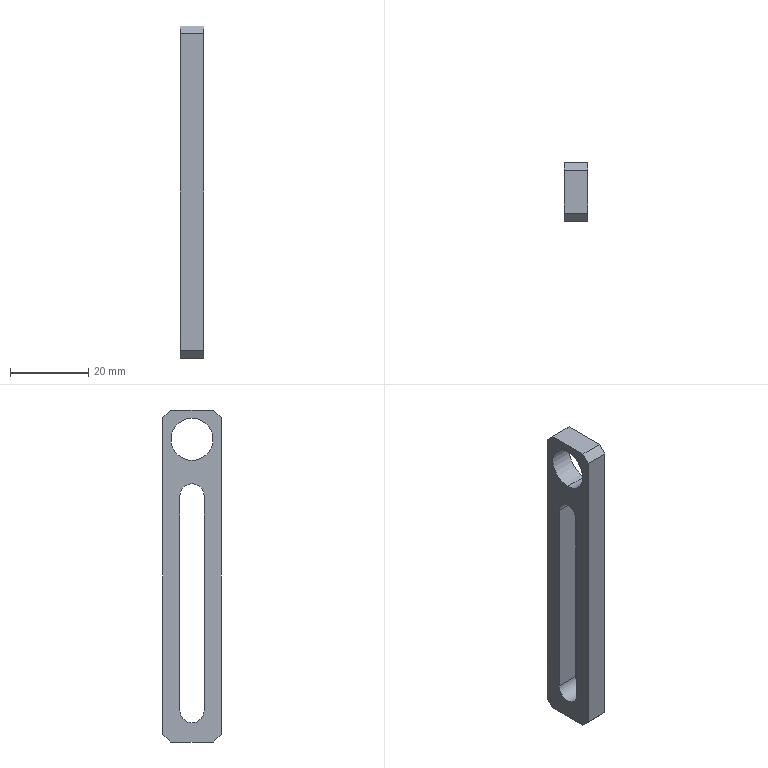Part | SolidWorks | features Chamfer 1, Extrusion 1, HoleWzd 1 | 1 solid | 17 faces | box 6 x 15 x 85 mm | volume 4825 mm3 | plane 12 | cylinder 5 | commonest cylinder face diameters 6.2 x3 10.8 x2
STEP:
#1=CARTESIAN_POINT('',(0.,-7.5,-2.1));
#2=VERTEX_POINT('',#1);
#3=CARTESIAN_POINT('',(0.,-7.5,-12.9));
#4=VERTEX_POINT('',#3);
#5=CARTESIAN_POINT('',(0.,-7.5,-7.5));
#6=DIRECTION('',(1.,0.,0.));
#7=DIRECTION('',(0.,0.,-1.));
#8=AXIS2_PLACEMENT_3D('',#5,#6,#7);
#9=CIRCLE('',#8,5.4);
#10=EDGE_CURVE('',#2,#4,#9,.T.);
#11=ORIENTED_EDGE('',*,*,#10,.F.);
#12=CARTESIAN_POINT('',(6.,-7.5,-2.1));
#13=VERTEX_POINT('',#12);
#14=CARTESIAN_POINT('',(6.,-7.5,-2.1));
#15=DIRECTION('',(1.,0.,0.));
#16=VECTOR('',#15,1000.);
#17=LINE('',#14,#16);
#18=EDGE_CURVE('',#2,#13,#17,.T.);
#19=ORIENTED_EDGE('',*,*,#18,.T.);
#20=CARTESIAN_POINT('',(6.,-7.5,-12.9));
#21=VERTEX_POINT('',#20);
#22=CARTESIAN_POINT('',(6.,-7.5,-7.5));
#23=DIRECTION('',(1.,0.,0.));
#24=DIRECTION('',(0.,0.,-1.));
#25=AXIS2_PLACEMENT_3D('',#22,#23,#24);
#26=CIRCLE('',#25,5.4);
#27=EDGE_CURVE('',#13,#21,#26,.T.);
#28=ORIENTED_EDGE('',*,*,#27,.T.);
#29=CARTESIAN_POINT('',(6.,-7.5,-12.9));
#30=DIRECTION('',(1.,0.,0.));
#31=VECTOR('',#30,1000.);
#32=LINE('',#29,#31);
#33=EDGE_CURVE('',#4,#21,#32,.T.);
#34=ORIENTED_EDGE('',*,*,#33,.F.);
#35=EDGE_LOOP('',(#11,#19,#28,#34));
#36=FACE_OUTER_BOUND('',#35,.T.);
#37=CARTESIAN_POINT('',(6.,-7.5,-7.5));
#38=DIRECTION('',(1.,0.,0.));
#39=DIRECTION('',(0.,0.,-1.));
#40=AXIS2_PLACEMENT_3D('',#37,#38,#39);
#41=CYLINDRICAL_SURFACE('',#40,5.4);
#42=ADVANCED_FACE('',(#36),#41,.F.);
#43=CARTESIAN_POINT('',(6.,-4.4,-22.));
#44=VERTEX_POINT('',#43);
#45=CARTESIAN_POINT('',(6.,-7.5,-18.9));
#46=VERTEX_POINT('',#45);
#47=CARTESIAN_POINT('',(6.,-7.5,-22.));
#48=DIRECTION('',(1.,0.,0.));
#49=DIRECTION('',(0.,0.,-1.));
#50=AXIS2_PLACEMENT_3D('',#47,#48,#49);
#51=CIRCLE('',#50,3.1);
#52=EDGE_CURVE('',#44,#46,#51,.T.);
#53=ORIENTED_EDGE('',*,*,#52,.T.);
#54=CARTESIAN_POINT('',(0.,-7.5,-18.9));
#55=VERTEX_POINT('',#54);
#56=CARTESIAN_POINT('',(6.,-7.5,-18.9));
#57=DIRECTION('',(-1.,0.,0.));
#58=VECTOR('',#57,1000.);
#59=LINE('',#56,#58);
#60=EDGE_CURVE('',#46,#55,#59,.T.);
#61=ORIENTED_EDGE('',*,*,#60,.T.);
#62=CARTESIAN_POINT('',(0.,-4.4,-22.));
#63=VERTEX_POINT('',#62);
#64=CARTESIAN_POINT('',(0.,-7.5,-22.));
#65=DIRECTION('',(1.,0.,0.));
#66=DIRECTION('',(0.,0.,-1.));
#67=AXIS2_PLACEMENT_3D('',#64,#65,#66);
#68=CIRCLE('',#67,3.1);
#69=EDGE_CURVE('',#63,#55,#68,.T.);
#70=ORIENTED_EDGE('',*,*,#69,.F.);
#71=CARTESIAN_POINT('',(6.,-4.4,-22.));
#72=DIRECTION('',(-1.,0.,0.));
#73=VECTOR('',#72,1000.);
#74=LINE('',#71,#73);
#75=EDGE_CURVE('',#44,#63,#74,.T.);
#76=ORIENTED_EDGE('',*,*,#75,.F.);
#77=EDGE_LOOP('',(#53,#61,#70,#76));
#78=FACE_OUTER_BOUND('',#77,.T.);
#79=CARTESIAN_POINT('',(6.,-7.5,-22.));
#80=DIRECTION('',(-1.,0.,0.));
#81=DIRECTION('',(0.,0.,1.));
#82=AXIS2_PLACEMENT_3D('',#79,#80,#81);
#83=CYLINDRICAL_SURFACE('',#82,3.1);
#84=ADVANCED_FACE('',(#78),#83,.F.);
#85=CARTESIAN_POINT('',(6.,-7.5,-7.5));
#86=DIRECTION('',(1.,0.,0.));
#87=DIRECTION('',(0.,0.,-1.));
#88=AXIS2_PLACEMENT_3D('',#85,#86,#87);
#89=CIRCLE('',#88,5.4);
#90=EDGE_CURVE('',#21,#13,#89,.T.);
#91=ORIENTED_EDGE('',*,*,#90,.F.);
#92=ORIENTED_EDGE('',*,*,#27,.F.);
#93=EDGE_LOOP('',(#91,#92));
#94=FACE_BOUND('',#93,.T.);
#95=CARTESIAN_POINT('',(6.,-13.,-85.));
#96=VERTEX_POINT('',#95);
#97=CARTESIAN_POINT('',(6.,-2.,-85.));
#98=VERTEX_POINT('',#97);
#99=CARTESIAN_POINT('',(6.,0.,-85.));
#100=DIRECTION('',(0.,1.,0.));
#101=VECTOR('',#100,1000.);
#102=LINE('',#99,#101);
#103=EDGE_CURVE('',#96,#98,#102,.T.);
#104=ORIENTED_EDGE('',*,*,#103,.T.);
#105=CARTESIAN_POINT('',(6.,0.,-83.));
#106=VERTEX_POINT('',#105);
#107=CARTESIAN_POINT('',(6.,34.,-49.));
#108=DIRECTION('',(0.,0.7071,0.7071));
#109=VECTOR('',#108,1000.);
#110=LINE('',#107,#109);
#111=EDGE_CURVE('',#98,#106,#110,.T.);
#112=ORIENTED_EDGE('',*,*,#111,.T.);
#113=CARTESIAN_POINT('',(6.,0.,-2.));
#114=VERTEX_POINT('',#113);
#115=CARTESIAN_POINT('',(6.,0.,0.));
#116=DIRECTION('',(0.,0.,1.));
#117=VECTOR('',#116,1000.);
#118=LINE('',#115,#117);
#119=EDGE_CURVE('',#106,#114,#118,.T.);
#120=ORIENTED_EDGE('',*,*,#119,.T.);
#121=CARTESIAN_POINT('',(6.,-2.,0.));
#122=VERTEX_POINT('',#121);
#123=CARTESIAN_POINT('',(6.,-8.5,6.5));
#124=DIRECTION('',(0.,-0.7071,0.7071));
#125=VECTOR('',#124,1000.);
#126=LINE('',#123,#125);
#127=EDGE_CURVE('',#114,#122,#126,.T.);
#128=ORIENTED_EDGE('',*,*,#127,.T.);
#129=CARTESIAN_POINT('',(6.,-13.,0.));
#130=VERTEX_POINT('',#129);
#131=CARTESIAN_POINT('',(6.,0.,0.));
#132=DIRECTION('',(0.,-1.,0.));
#133=VECTOR('',#132,1000.);
#134=LINE('',#131,#133);
#135=EDGE_CURVE('',#122,#130,#134,.T.);
#136=ORIENTED_EDGE('',*,*,#135,.T.);
#137=CARTESIAN_POINT('',(6.,-15.,-2.));
#138=VERTEX_POINT('',#137);
#139=CARTESIAN_POINT('',(6.,-14.,-1.));
#140=DIRECTION('',(0.,-0.7071,-0.7071));
#141=VECTOR('',#140,1000.);
#142=LINE('',#139,#141);
#143=EDGE_CURVE('',#130,#138,#142,.T.);
#144=ORIENTED_EDGE('',*,*,#143,.T.);
#145=CARTESIAN_POINT('',(6.,-15.,-83.));
#146=VERTEX_POINT('',#145);
#147=CARTESIAN_POINT('',(6.,-15.,0.));
#148=DIRECTION('',(0.,0.,-1.));
#149=VECTOR('',#148,1000.);
#150=LINE('',#147,#149);
#151=EDGE_CURVE('',#138,#146,#150,.T.);
#152=ORIENTED_EDGE('',*,*,#151,.T.);
#153=CARTESIAN_POINT('',(6.,-56.5,-41.5));
#154=DIRECTION('',(0.,0.7071,-0.7071));
#155=VECTOR('',#154,1000.);
#156=LINE('',#153,#155);
#157=EDGE_CURVE('',#146,#96,#156,.T.);
#158=ORIENTED_EDGE('',*,*,#157,.T.);
#159=EDGE_LOOP('',(#104,#112,#120,#128,#136,#144,#152,#158));
#160=FACE_OUTER_BOUND('',#159,.T.);
#161=CARTESIAN_POINT('',(6.,-10.6,-22.));
#162=VERTEX_POINT('',#161);
#163=CARTESIAN_POINT('',(6.,-10.6,-77.));
#164=VERTEX_POINT('',#163);
#165=CARTESIAN_POINT('',(6.,-10.6,-22.));
#166=DIRECTION('',(0.,0.,-1.));
#167=VECTOR('',#166,1000.);
#168=LINE('',#165,#167);
#169=EDGE_CURVE('',#162,#164,#168,.T.);
#170=ORIENTED_EDGE('',*,*,#169,.F.);
#171=CARTESIAN_POINT('',(6.,-7.5,-22.));
#172=DIRECTION('',(1.,0.,0.));
#173=DIRECTION('',(0.,0.,-1.));
#174=AXIS2_PLACEMENT_3D('',#171,#172,#173);
#175=CIRCLE('',#174,3.1);
#176=EDGE_CURVE('',#46,#162,#175,.T.);
#177=ORIENTED_EDGE('',*,*,#176,.F.);
#178=ORIENTED_EDGE('',*,*,#52,.F.);
#179=CARTESIAN_POINT('',(6.,-4.4,-77.));
#180=VERTEX_POINT('',#179);
#181=CARTESIAN_POINT('',(6.,-4.4,-22.));
#182=DIRECTION('',(0.,0.,1.));
#183=VECTOR('',#182,1000.);
#184=LINE('',#181,#183);
#185=EDGE_CURVE('',#180,#44,#184,.T.);
#186=ORIENTED_EDGE('',*,*,#185,.F.);
#187=CARTESIAN_POINT('',(6.,-7.5,-77.));
#188=DIRECTION('',(1.,0.,0.));
#189=DIRECTION('',(0.,0.,-1.));
#190=AXIS2_PLACEMENT_3D('',#187,#188,#189);
#191=CIRCLE('',#190,3.1);
#192=EDGE_CURVE('',#164,#180,#191,.T.);
#193=ORIENTED_EDGE('',*,*,#192,.F.);
#194=EDGE_LOOP('',(#170,#177,#178,#186,#193));
#195=FACE_BOUND('',#194,.T.);
#196=CARTESIAN_POINT('',(6.,-15.,0.));
#197=DIRECTION('',(1.,0.,0.));
#198=DIRECTION('',(0.,0.,-1.));
#199=AXIS2_PLACEMENT_3D('',#196,#197,#198);
#200=PLANE('',#199);
#201=ADVANCED_FACE('',(#94,#160,#195),#200,.T.);
#202=CARTESIAN_POINT('',(0.,-7.5,-7.5));
#203=DIRECTION('',(1.,0.,0.));
#204=DIRECTION('',(0.,0.,-1.));
#205=AXIS2_PLACEMENT_3D('',#202,#203,#204);
#206=CIRCLE('',#205,5.4);
#207=EDGE_CURVE('',#4,#2,#206,.T.);
#208=ORIENTED_EDGE('',*,*,#207,.T.);
#209=ORIENTED_EDGE('',*,*,#10,.T.);
#210=EDGE_LOOP('',(#208,#209));
#211=FACE_BOUND('',#210,.T.);
#212=CARTESIAN_POINT('',(0.,0.,-83.));
#213=VERTEX_POINT('',#212);
#214=CARTESIAN_POINT('',(0.,0.,-2.));
#215=VERTEX_POINT('',#214);
#216=CARTESIAN_POINT('',(0.,0.,0.));
#217=DIRECTION('',(0.,0.,1.));
#218=VECTOR('',#217,1000.);
#219=LINE('',#216,#218);
#220=EDGE_CURVE('',#213,#215,#219,.T.);
#221=ORIENTED_EDGE('',*,*,#220,.F.);
#222=CARTESIAN_POINT('',(0.,-2.,-85.));
#223=VERTEX_POINT('',#222);
#224=CARTESIAN_POINT('',(0.,0.,-83.));
#225=DIRECTION('',(0.,-0.7071,-0.7071));
#226=VECTOR('',#225,1000.);
#227=LINE('',#224,#226);
#228=EDGE_CURVE('',#213,#223,#227,.T.);
#229=ORIENTED_EDGE('',*,*,#228,.T.);
#230=CARTESIAN_POINT('',(0.,-13.,-85.));
#231=VERTEX_POINT('',#230);
#232=CARTESIAN_POINT('',(0.,0.,-85.));
#233=DIRECTION('',(0.,1.,0.));
#234=VECTOR('',#233,1000.);
#235=LINE('',#232,#234);
#236=EDGE_CURVE('',#231,#223,#235,.T.);
#237=ORIENTED_EDGE('',*,*,#236,.F.);
#238=CARTESIAN_POINT('',(0.,-15.,-83.));
#239=VERTEX_POINT('',#238);
#240=CARTESIAN_POINT('',(0.,-13.,-85.));
#241=DIRECTION('',(0.,-0.7071,0.7071));
#242=VECTOR('',#241,1000.);
#243=LINE('',#240,#242);
#244=EDGE_CURVE('',#231,#239,#243,.T.);
#245=ORIENTED_EDGE('',*,*,#244,.T.);
#246=CARTESIAN_POINT('',(0.,-15.,-2.));
#247=VERTEX_POINT('',#246);
#248=CARTESIAN_POINT('',(0.,-15.,0.));
#249=DIRECTION('',(0.,0.,-1.));
#250=VECTOR('',#249,1000.);
#251=LINE('',#248,#250);
#252=EDGE_CURVE('',#247,#239,#251,.T.);
#253=ORIENTED_EDGE('',*,*,#252,.F.);
#254=CARTESIAN_POINT('',(0.,-13.,0.));
#255=VERTEX_POINT('',#254);
#256=CARTESIAN_POINT('',(0.,-15.,-2.));
#257=DIRECTION('',(0.,0.7071,0.7071));
#258=VECTOR('',#257,1000.);
#259=LINE('',#256,#258);
#260=EDGE_CURVE('',#247,#255,#259,.T.);
#261=ORIENTED_EDGE('',*,*,#260,.T.);
#262=CARTESIAN_POINT('',(0.,-2.,0.));
#263=VERTEX_POINT('',#262);
#264=CARTESIAN_POINT('',(0.,0.,0.));
#265=DIRECTION('',(0.,-1.,0.));
#266=VECTOR('',#265,1000.);
#267=LINE('',#264,#266);
#268=EDGE_CURVE('',#263,#255,#267,.T.);
#269=ORIENTED_EDGE('',*,*,#268,.F.);
#270=CARTESIAN_POINT('',(0.,-2.,0.));
#271=DIRECTION('',(0.,0.7071,-0.7071));
#272=VECTOR('',#271,1000.);
#273=LINE('',#270,#272);
#274=EDGE_CURVE('',#263,#215,#273,.T.);
#275=ORIENTED_EDGE('',*,*,#274,.T.);
#276=EDGE_LOOP('',(#221,#229,#237,#245,#253,#261,#269,#275));
#277=FACE_OUTER_BOUND('',#276,.T.);
#278=ORIENTED_EDGE('',*,*,#69,.T.);
#279=CARTESIAN_POINT('',(0.,-10.6,-22.));
#280=VERTEX_POINT('',#279);
#281=CARTESIAN_POINT('',(0.,-7.5,-22.));
#282=DIRECTION('',(1.,0.,0.));
#283=DIRECTION('',(0.,0.,-1.));
#284=AXIS2_PLACEMENT_3D('',#281,#282,#283);
#285=CIRCLE('',#284,3.1);
#286=EDGE_CURVE('',#55,#280,#285,.T.);
#287=ORIENTED_EDGE('',*,*,#286,.T.);
#288=CARTESIAN_POINT('',(0.,-10.6,-77.));
#289=VERTEX_POINT('',#288);
#290=CARTESIAN_POINT('',(0.,-10.6,-22.));
#291=DIRECTION('',(0.,0.,-1.));
#292=VECTOR('',#291,1000.);
#293=LINE('',#290,#292);
#294=EDGE_CURVE('',#280,#289,#293,.T.);
#295=ORIENTED_EDGE('',*,*,#294,.T.);
#296=CARTESIAN_POINT('',(0.,-4.4,-77.));
#297=VERTEX_POINT('',#296);
#298=CARTESIAN_POINT('',(0.,-7.5,-77.));
#299=DIRECTION('',(1.,0.,0.));
#300=DIRECTION('',(0.,0.,-1.));
#301=AXIS2_PLACEMENT_3D('',#298,#299,#300);
#302=CIRCLE('',#301,3.1);
#303=EDGE_CURVE('',#289,#297,#302,.T.);
#304=ORIENTED_EDGE('',*,*,#303,.T.);
#305=CARTESIAN_POINT('',(0.,-4.4,-22.));
#306=DIRECTION('',(0.,0.,1.));
#307=VECTOR('',#306,1000.);
#308=LINE('',#305,#307);
#309=EDGE_CURVE('',#297,#63,#308,.T.);
#310=ORIENTED_EDGE('',*,*,#309,.T.);
#311=EDGE_LOOP('',(#278,#287,#295,#304,#310));
#312=FACE_BOUND('',#311,.T.);
#313=CARTESIAN_POINT('',(0.,-15.,0.));
#314=DIRECTION('',(1.,0.,0.));
#315=DIRECTION('',(0.,0.,-1.));
#316=AXIS2_PLACEMENT_3D('',#313,#314,#315);
#317=PLANE('',#316);
#318=ADVANCED_FACE('',(#211,#277,#312),#317,.F.);
#319=ORIENTED_EDGE('',*,*,#268,.T.);
#320=CARTESIAN_POINT('',(6.,-13.,0.));
#321=DIRECTION('',(1.,0.,0.));
#322=VECTOR('',#321,1000.);
#323=LINE('',#320,#322);
#324=EDGE_CURVE('',#255,#130,#323,.T.);
#325=ORIENTED_EDGE('',*,*,#324,.T.);
#326=ORIENTED_EDGE('',*,*,#135,.F.);
#327=CARTESIAN_POINT('',(6.,-2.,0.));
#328=DIRECTION('',(-1.,0.,0.));
#329=VECTOR('',#328,1000.);
#330=LINE('',#327,#329);
#331=EDGE_CURVE('',#122,#263,#330,.T.);
#332=ORIENTED_EDGE('',*,*,#331,.T.);
#333=EDGE_LOOP('',(#319,#325,#326,#332));
#334=FACE_OUTER_BOUND('',#333,.T.);
#335=CARTESIAN_POINT('',(6.,0.,0.));
#336=DIRECTION('',(0.,0.,-1.));
#337=DIRECTION('',(0.,1.,0.));
#338=AXIS2_PLACEMENT_3D('',#335,#336,#337);
#339=PLANE('',#338);
#340=ADVANCED_FACE('',(#334),#339,.F.);
#341=ORIENTED_EDGE('',*,*,#252,.T.);
#342=CARTESIAN_POINT('',(6.,-15.,-83.));
#343=DIRECTION('',(1.,0.,0.));
#344=VECTOR('',#343,1000.);
#345=LINE('',#342,#344);
#346=EDGE_CURVE('',#239,#146,#345,.T.);
#347=ORIENTED_EDGE('',*,*,#346,.T.);
#348=ORIENTED_EDGE('',*,*,#151,.F.);
#349=CARTESIAN_POINT('',(6.,-15.,-2.));
#350=DIRECTION('',(-1.,0.,0.));
#351=VECTOR('',#350,1000.);
#352=LINE('',#349,#351);
#353=EDGE_CURVE('',#138,#247,#352,.T.);
#354=ORIENTED_EDGE('',*,*,#353,.T.);
#355=EDGE_LOOP('',(#341,#347,#348,#354));
#356=FACE_OUTER_BOUND('',#355,.T.);
#357=CARTESIAN_POINT('',(6.,-15.,0.));
#358=DIRECTION('',(0.,1.,0.));
#359=DIRECTION('',(0.,0.,1.));
#360=AXIS2_PLACEMENT_3D('',#357,#358,#359);
#361=PLANE('',#360);
#362=ADVANCED_FACE('',(#356),#361,.F.);
#363=ORIENTED_EDGE('',*,*,#236,.T.);
#364=CARTESIAN_POINT('',(6.,-2.,-85.));
#365=DIRECTION('',(1.,0.,0.));
#366=VECTOR('',#365,1000.);
#367=LINE('',#364,#366);
#368=EDGE_CURVE('',#223,#98,#367,.T.);
#369=ORIENTED_EDGE('',*,*,#368,.T.);
#370=ORIENTED_EDGE('',*,*,#103,.F.);
#371=CARTESIAN_POINT('',(6.,-13.,-85.));
#372=DIRECTION('',(-1.,0.,0.));
#373=VECTOR('',#372,1000.);
#374=LINE('',#371,#373);
#375=EDGE_CURVE('',#96,#231,#374,.T.);
#376=ORIENTED_EDGE('',*,*,#375,.T.);
#377=EDGE_LOOP('',(#363,#369,#370,#376));
#378=FACE_OUTER_BOUND('',#377,.T.);
#379=CARTESIAN_POINT('',(6.,0.,-85.));
#380=DIRECTION('',(0.,0.,1.));
#381=DIRECTION('',(1.,0.,0.));
#382=AXIS2_PLACEMENT_3D('',#379,#380,#381);
#383=PLANE('',#382);
#384=ADVANCED_FACE('',(#378),#383,.F.);
#385=ORIENTED_EDGE('',*,*,#119,.F.);
#386=CARTESIAN_POINT('',(6.,0.,-83.));
#387=DIRECTION('',(-1.,0.,0.));
#388=VECTOR('',#387,1000.);
#389=LINE('',#386,#388);
#390=EDGE_CURVE('',#106,#213,#389,.T.);
#391=ORIENTED_EDGE('',*,*,#390,.T.);
#392=ORIENTED_EDGE('',*,*,#220,.T.);
#393=CARTESIAN_POINT('',(6.,0.,-2.));
#394=DIRECTION('',(1.,0.,0.));
#395=VECTOR('',#394,1000.);
#396=LINE('',#393,#395);
#397=EDGE_CURVE('',#215,#114,#396,.T.);
#398=ORIENTED_EDGE('',*,*,#397,.T.);
#399=EDGE_LOOP('',(#385,#391,#392,#398));
#400=FACE_OUTER_BOUND('',#399,.T.);
#401=CARTESIAN_POINT('',(6.,0.,0.));
#402=DIRECTION('',(0.,-1.,0.));
#403=DIRECTION('',(0.,0.,-1.));
#404=AXIS2_PLACEMENT_3D('',#401,#402,#403);
#405=PLANE('',#404);
#406=ADVANCED_FACE('',(#400),#405,.F.);
#407=ORIENTED_EDGE('',*,*,#60,.F.);
#408=ORIENTED_EDGE('',*,*,#176,.T.);
#409=CARTESIAN_POINT('',(6.,-10.6,-22.));
#410=DIRECTION('',(-1.,0.,0.));
#411=VECTOR('',#410,1000.);
#412=LINE('',#409,#411);
#413=EDGE_CURVE('',#162,#280,#412,.T.);
#414=ORIENTED_EDGE('',*,*,#413,.T.);
#415=ORIENTED_EDGE('',*,*,#286,.F.);
#416=EDGE_LOOP('',(#407,#408,#414,#415));
#417=FACE_OUTER_BOUND('',#416,.T.);
#418=CARTESIAN_POINT('',(6.,-7.5,-22.));
#419=DIRECTION('',(-1.,0.,0.));
#420=DIRECTION('',(0.,0.,1.));
#421=AXIS2_PLACEMENT_3D('',#418,#419,#420);
#422=CYLINDRICAL_SURFACE('',#421,3.1);
#423=ADVANCED_FACE('',(#417),#422,.F.);
#424=ORIENTED_EDGE('',*,*,#294,.F.);
#425=ORIENTED_EDGE('',*,*,#413,.F.);
#426=ORIENTED_EDGE('',*,*,#169,.T.);
#427=CARTESIAN_POINT('',(6.,-10.6,-77.));
#428=DIRECTION('',(-1.,0.,0.));
#429=VECTOR('',#428,1000.);
#430=LINE('',#427,#429);
#431=EDGE_CURVE('',#164,#289,#430,.T.);
#432=ORIENTED_EDGE('',*,*,#431,.T.);
#433=EDGE_LOOP('',(#424,#425,#426,#432));
#434=FACE_OUTER_BOUND('',#433,.T.);
#435=CARTESIAN_POINT('',(6.,-10.6,-22.));
#436=DIRECTION('',(0.,1.,0.));
#437=DIRECTION('',(0.,0.,1.));
#438=AXIS2_PLACEMENT_3D('',#435,#436,#437);
#439=PLANE('',#438);
#440=ADVANCED_FACE('',(#434),#439,.T.);
#441=ORIENTED_EDGE('',*,*,#303,.F.);
#442=ORIENTED_EDGE('',*,*,#431,.F.);
#443=ORIENTED_EDGE('',*,*,#192,.T.);
#444=CARTESIAN_POINT('',(6.,-4.4,-77.));
#445=DIRECTION('',(-1.,0.,0.));
#446=VECTOR('',#445,1000.);
#447=LINE('',#444,#446);
#448=EDGE_CURVE('',#180,#297,#447,.T.);
#449=ORIENTED_EDGE('',*,*,#448,.T.);
#450=EDGE_LOOP('',(#441,#442,#443,#449));
#451=FACE_OUTER_BOUND('',#450,.T.);
#452=CARTESIAN_POINT('',(6.,-7.5,-77.));
#453=DIRECTION('',(-1.,0.,0.));
#454=DIRECTION('',(0.,0.,1.));
#455=AXIS2_PLACEMENT_3D('',#452,#453,#454);
#456=CYLINDRICAL_SURFACE('',#455,3.1);
#457=ADVANCED_FACE('',(#451),#456,.F.);
#458=ORIENTED_EDGE('',*,*,#309,.F.);
#459=ORIENTED_EDGE('',*,*,#448,.F.);
#460=ORIENTED_EDGE('',*,*,#185,.T.);
#461=ORIENTED_EDGE('',*,*,#75,.T.);
#462=EDGE_LOOP('',(#458,#459,#460,#461));
#463=FACE_OUTER_BOUND('',#462,.T.);
#464=CARTESIAN_POINT('',(6.,-4.4,-22.));
#465=DIRECTION('',(0.,-1.,0.));
#466=DIRECTION('',(0.,0.,-1.));
#467=AXIS2_PLACEMENT_3D('',#464,#465,#466);
#468=PLANE('',#467);
#469=ADVANCED_FACE('',(#463),#468,.T.);
#470=ORIENTED_EDGE('',*,*,#18,.F.);
#471=ORIENTED_EDGE('',*,*,#207,.F.);
#472=ORIENTED_EDGE('',*,*,#33,.T.);
#473=ORIENTED_EDGE('',*,*,#90,.T.);
#474=EDGE_LOOP('',(#470,#471,#472,#473));
#475=FACE_OUTER_BOUND('',#474,.T.);
#476=CARTESIAN_POINT('',(6.,-7.5,-7.5));
#477=DIRECTION('',(1.,0.,0.));
#478=DIRECTION('',(0.,0.,-1.));
#479=AXIS2_PLACEMENT_3D('',#476,#477,#478);
#480=CYLINDRICAL_SURFACE('',#479,5.4);
#481=ADVANCED_FACE('',(#475),#480,.F.);
#482=ORIENTED_EDGE('',*,*,#111,.F.);
#483=ORIENTED_EDGE('',*,*,#368,.F.);
#484=ORIENTED_EDGE('',*,*,#228,.F.);
#485=ORIENTED_EDGE('',*,*,#390,.F.);
#486=EDGE_LOOP('',(#482,#483,#484,#485));
#487=FACE_OUTER_BOUND('',#486,.T.);
#488=CARTESIAN_POINT('',(6.,0.,-83.));
#489=DIRECTION('',(0.,-0.7071,0.7071));
#490=DIRECTION('',(0.,-0.7071,-0.7071));
#491=AXIS2_PLACEMENT_3D('',#488,#489,#490);
#492=PLANE('',#491);
#493=ADVANCED_FACE('',(#487),#492,.F.);
#494=ORIENTED_EDGE('',*,*,#157,.F.);
#495=ORIENTED_EDGE('',*,*,#346,.F.);
#496=ORIENTED_EDGE('',*,*,#244,.F.);
#497=ORIENTED_EDGE('',*,*,#375,.F.);
#498=EDGE_LOOP('',(#494,#495,#496,#497));
#499=FACE_OUTER_BOUND('',#498,.T.);
#500=CARTESIAN_POINT('',(6.,-13.,-85.));
#501=DIRECTION('',(0.,0.7071,0.7071));
#502=DIRECTION('',(0.,-0.7071,0.7071));
#503=AXIS2_PLACEMENT_3D('',#500,#501,#502);
#504=PLANE('',#503);
#505=ADVANCED_FACE('',(#499),#504,.F.);
#506=ORIENTED_EDGE('',*,*,#143,.F.);
#507=ORIENTED_EDGE('',*,*,#324,.F.);
#508=ORIENTED_EDGE('',*,*,#260,.F.);
#509=ORIENTED_EDGE('',*,*,#353,.F.);
#510=EDGE_LOOP('',(#506,#507,#508,#509));
#511=FACE_OUTER_BOUND('',#510,.T.);
#512=CARTESIAN_POINT('',(6.,-15.,-2.));
#513=DIRECTION('',(0.,0.7071,-0.7071));
#514=DIRECTION('',(0.,0.7071,0.7071));
#515=AXIS2_PLACEMENT_3D('',#512,#513,#514);
#516=PLANE('',#515);
#517=ADVANCED_FACE('',(#511),#516,.F.);
#518=ORIENTED_EDGE('',*,*,#127,.F.);
#519=ORIENTED_EDGE('',*,*,#397,.F.);
#520=ORIENTED_EDGE('',*,*,#274,.F.);
#521=ORIENTED_EDGE('',*,*,#331,.F.);
#522=EDGE_LOOP('',(#518,#519,#520,#521));
#523=FACE_OUTER_BOUND('',#522,.T.);
#524=CARTESIAN_POINT('',(6.,-2.,0.));
#525=DIRECTION('',(0.,-0.7071,-0.7071));
#526=DIRECTION('',(0.,0.7071,-0.7071));
#527=AXIS2_PLACEMENT_3D('',#524,#525,#526);
#528=PLANE('',#527);
#529=ADVANCED_FACE('',(#523),#528,.F.);
#530=CLOSED_SHELL('',(#42,#84,#201,#318,#340,#362,#384,#406,#423,#440,#457,#469,#481,#493,#505,#517,#529));
#531=MANIFOLD_SOLID_BREP('',#530);
#532=CARTESIAN_POINT('',(0.,0.,0.));
#533=DIRECTION('',(0.,0.,1.));
#534=DIRECTION('',(1.,0.,0.));
#535=AXIS2_PLACEMENT_3D('',#532,#533,#534);
#536=(LENGTH_UNIT()NAMED_UNIT(*)SI_UNIT(.MILLI.,.METRE.));
#537=UNCERTAINTY_MEASURE_WITH_UNIT(LENGTH_MEASURE(0.00001),#536,'','');
#538=(NAMED_UNIT(*)PLANE_ANGLE_UNIT()SI_UNIT($,.RADIAN.));
#539=(NAMED_UNIT(*)SI_UNIT($,.STERADIAN.)SOLID_ANGLE_UNIT());
#540=(GEOMETRIC_REPRESENTATION_CONTEXT(3)GLOBAL_UNCERTAINTY_ASSIGNED_CONTEXT((#537))GLOBAL_UNIT_ASSIGNED_CONTEXT((#536,#538,#539))REPRESENTATION_CONTEXT('',''));
#541=ADVANCED_BREP_SHAPE_REPRESENTATION('',(#531,#535),#540);